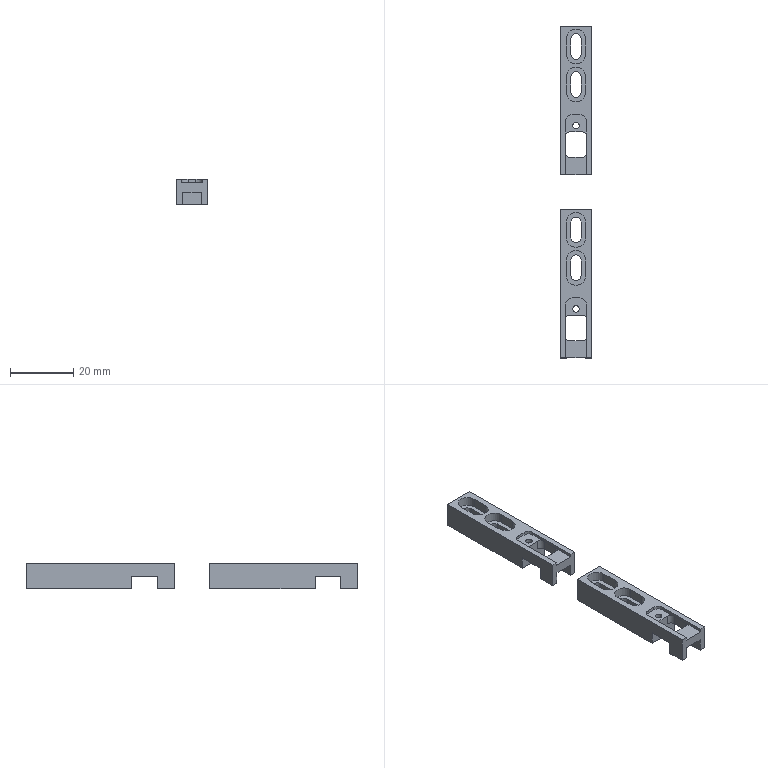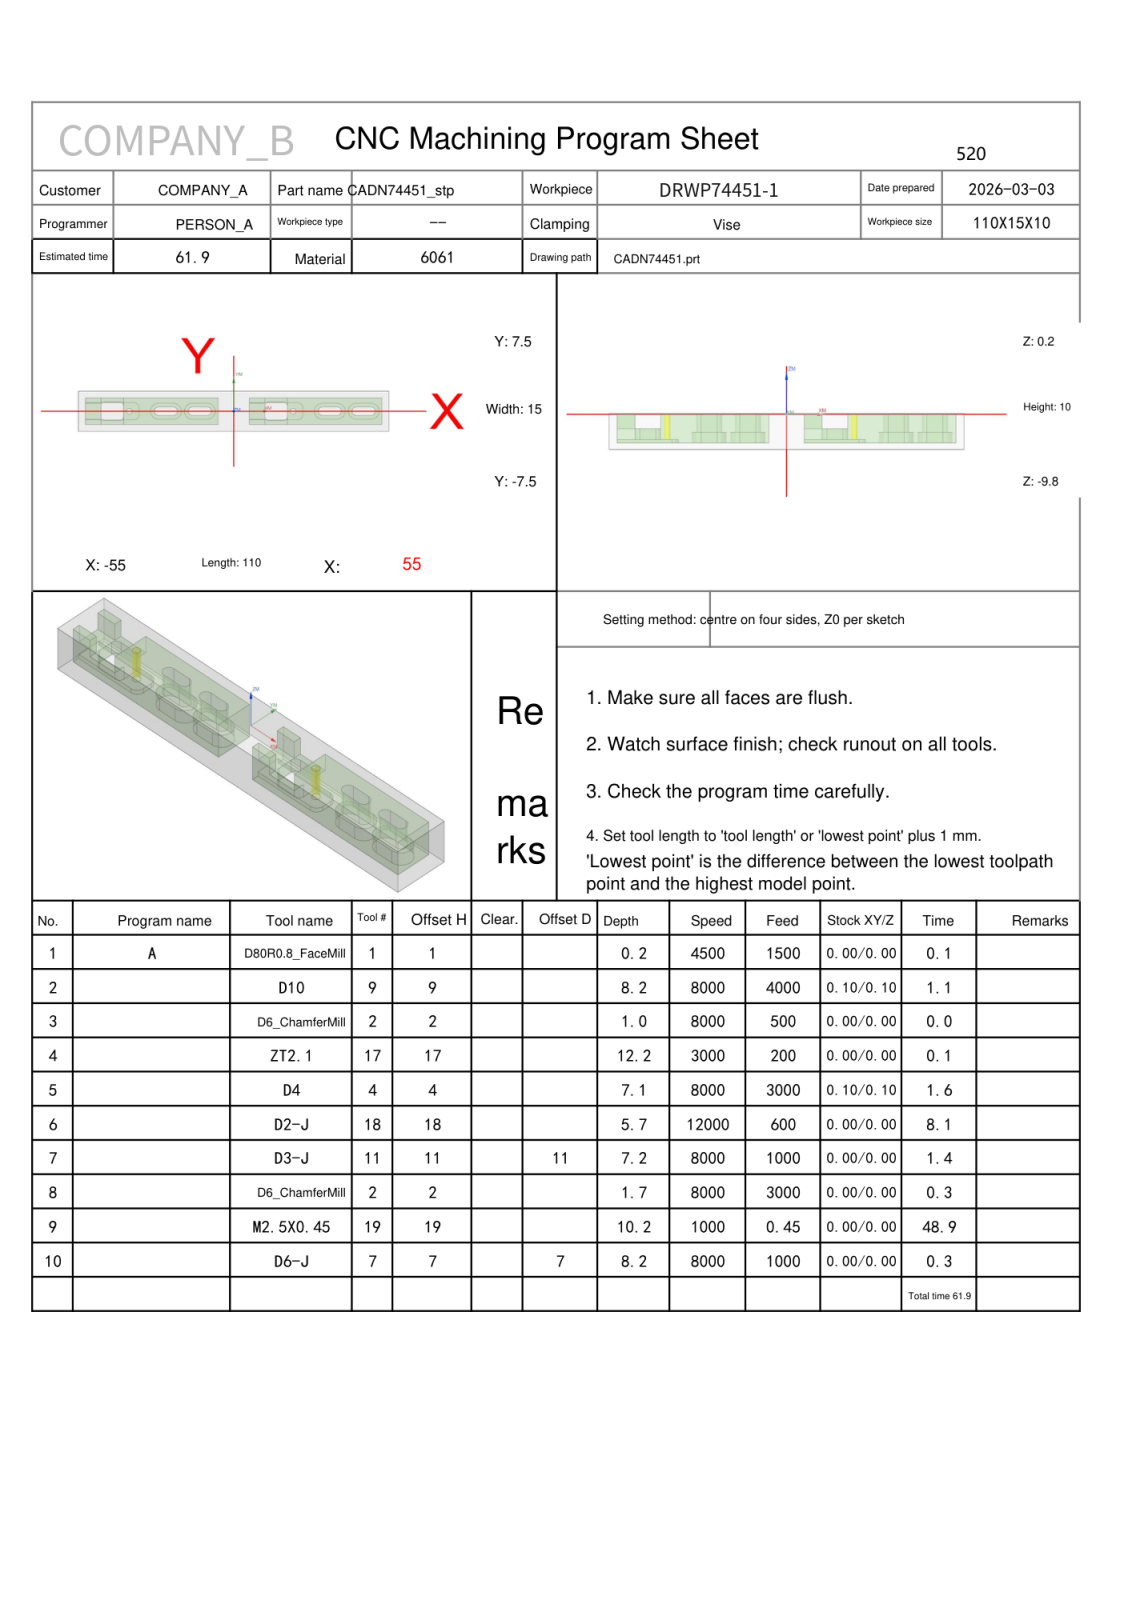NC program | NX | posted by the shop | part box 10 x 105 x 8 mm
Lines 4175 to 4761 of 4761:
N7 T11 M06
(D3-J  D=3. R=0. H=11 ce=0.00 di=0.00)
G00 G90 G54 X17.5 Y1.409 M03 S8000
G43 H11 Z50.
M08
Z.5
G01 Y2. Z.469 F600.
X12.5 Z.207
Y-1.95 Z0.0
G41 D11
Y-2.
X17.5 Z-.139
Y2. Z-.25
X12.5 Z-.389
Y-2. Z-.5
X17.5 Z-.639
Y2. Z-.75
X12.5 Z-.889
Y-2. Z-1.
X17.5 Z-1.139
Y2. Z-1.25
X12.5 Z-1.389
Y-2. Z-1.5
X17.5 Z-1.639
Y2. Z-1.75
X12.5 Z-1.889
Y-2. Z-2.
X17.5 Z-2.139
Y2. Z-2.25
X12.5 Z-2.389
Y-2. Z-2.5
X17.5 Z-2.639
Y2. Z-2.75
X12.5 Z-2.889
Y-2. Z-3.
X17.5 Z-3.139
Y2. Z-3.25
X12.5 Z-3.389
Y-2. Z-3.5
X17.5 Z-3.639
Y2. Z-3.75
X12.5 Z-3.889
Y-2. Z-4.
X17.5 Z-4.139
Y2. Z-4.25
X12.5 Z-4.389
Y-2. Z-4.5
X17.5 Z-4.639
Y2. Z-4.75
X12.5 Z-4.889
Y-2. Z-5.
X17.5 Z-5.139
Y2. Z-5.25
X12.5 Z-5.389
Y-2. Z-5.5
X17.5 Z-5.639
Y2. Z-5.75
X12.5 Z-5.889
Y-2. Z-6.
X17.5 Z-6.139
Y2. Z-6.25
X12.5 Z-6.389
Y-2. Z-6.5
X17.5 Z-6.639
Y2. Z-6.75
X12.5 Z-6.889
Y-2. Z-7.
X17.5
Y2.
X12.5
Y-2.
X12.9
X12.928 Y-1.998
X12.948 Y-1.978
X12.95 Y-1.95
G40 Y-1.9
Z-6.
G00 Z50.
X-45.5 Y-1.409
Z.5
G01 Y-2. Z.469
X-40.5 Z.207
Y1.95 Z0.0
G41 D11
Y2.
X-45.5 Z-.139
Y-2. Z-.25
X-40.5 Z-.389
Y2. Z-.5
X-45.5 Z-.639
Y-2. Z-.75
X-40.5 Z-.889
Y2. Z-1.
X-45.5 Z-1.139
Y-2. Z-1.25
X-40.5 Z-1.389
Y2. Z-1.5
X-45.5 Z-1.639
Y-2. Z-1.75
X-40.5 Z-1.889
Y2. Z-2.
X-45.5 Z-2.139
Y-2. Z-2.25
X-40.5 Z-2.389
Y2. Z-2.5
X-45.5 Z-2.639
Y-2. Z-2.75
X-40.5 Z-2.889
Y2. Z-3.
X-45.5 Z-3.139
Y-2. Z-3.25
X-40.5 Z-3.389
Y2. Z-3.5
X-45.5 Z-3.639
Y-2. Z-3.75
X-40.5 Z-3.889
Y2. Z-4.
X-45.5 Z-4.139
Y-2. Z-4.25
X-40.5 Z-4.389
Y2. Z-4.5
X-45.5 Z-4.639
Y-2. Z-4.75
X-40.5 Z-4.889
Y2. Z-5.
X-45.5 Z-5.139
Y-2. Z-5.25
X-40.5 Z-5.389
Y2. Z-5.5
X-45.5 Z-5.639
Y-2. Z-5.75
X-40.5 Z-5.889
Y2. Z-6.
X-45.5 Z-6.139
Y-2. Z-6.25
X-40.5 Z-6.389
Y2. Z-6.5
X-45.5 Z-6.639
Y-2. Z-6.75
X-40.5 Z-6.889
Y2. Z-7.
X-45.5
Y-2.
X-40.5
Y2.
X-40.9
X-40.928 Y1.998
X-40.948 Y1.978
X-40.95 Y1.95
G40 Y1.9
Z-6.
G00 Z50.
G00 G90 X-43. Y9.8 M03 S8000
Z50.
Z-3.5
G01 Z-4. F1000.
Y5.3
X-40.8
Y3.2
X-45.2
Y5.3
X-43.
X-42.5
Y9.8
Z-3.5
G00 Z50.
X-57.3 Y0.0
Z-3.5
G01 Z-4.
X-52.8
Y1.2
X-46.7
Y-1.2
X-52.8
Y0.0
Y.5
X-57.3
Z-3.5
G00 Z50.
X-43. Y-9.8
Z-3.5
G01 Z-4.
Y-5.3
X-45.2
Y-3.2
X-40.8
Y-5.3
X-43.
X-43.5
Y-9.8
Z-3.5
G00 Z50.
X15. Y9.8
Z-3.5
G01 Z-4.
Y5.3
X17.2
Y3.2
X12.8
Y5.3
X15.
X15.5
Y9.8
Z-3.5
G00 Z50.
X13.1
Z-3.5
G01 Z-4.
Y0.0
X11.3
Y-1.2
X5.2
Y1.2
X11.3
Y0.0
Y-.5
X13.1
Y-9.8
Z-3.5
G00 Z50.
X15.
Z-3.5
G01 Z-4.
Y-5.3
X12.8
Y-3.2
X17.2
Y-5.3
X15.
X14.5
Y-9.8
Z-3.5
G00 Z50.
G00 G90 X16.4 Y-7.35 M03 S8000
Z50.
Z-3.495
G01 Z-3.995 F1000.
G41 D11
X16.5
G03 X17.5 Y-6.35 I0.0 J1.
G01 Y6.35
G03 X16.5 Y7.35 I-1. J0.0
G01 G40 X16.4
Z-3.495
G00 Z50.
X13.6
Z-3.495
G01 Z-3.995
G41 D11
X13.5
G03 X12.5 Y6.35 I0.0 J-1.
G01 Y1.5
X4.15
G03 X3.15 Y.5 I0.0 J-1.
G01 G40 Y.4
Y-.4
G41 D11
Y-.5
G03 X4.15 Y-1.5 I1. J0.0
G01 X12.5
Y-6.35
G03 X13.5 Y-7.35 I1. J0.0
G01 G40 X13.6
Z-3.495
G00 Z50.
X-41.6
Z-3.495
G01 Z-3.995
G41 D11
X-41.5
G03 X-40.5 Y-6.35 I0.0 J1.
G01 Y6.35
G03 X-41.5 Y7.35 I-1. J0.0
G01 G40 X-41.6
Z-3.495
G00 Z50.
X-44.4
Z-3.495
G01 Z-3.995
G41 D11
X-44.5
G03 X-45.5 Y6.35 I0.0 J-1.
G01 Y1.5
X-53.85
G03 X-54.85 Y.5 I0.0 J-1.
G01 G40 Y.4
Y-.4
G41 D11
Y-.5
G03 X-53.85 Y-1.5 I1. J0.0
G01 X-45.5
Y-6.35
G03 X-44.5 Y-7.35 I1. J0.0
G01 G40 X-44.4
Z-3.495
G00 Z50.
G91 G28 Z0.0
M05
M09
G91 G28 Z0.0
M01
N8 T02 M06
(D6_ChamferMill  D=6. R=0. H=02 ce=0.00 di=0.00)
G00 G90 G54 X36. Y-7.128 M03 S8000
G43 H02 Z50.
M08
Z2.099
G01 Z-1.5 F3000.
G03 X36.08 Y-6.828 I-.52 J.3
X35.78 Y-6.308 I-.6 J0.0
G01 X35.75 Y-6.3
X19.
G02 X17.7 Y-5. I0.0 J1.3
G01 Y5.
G02 X19. Y6.3 I1.3 J0.0
G01 X52.5
G02 X53.8 Y5. I0.0 J-1.3
G01 Y-5.
G02 X52.5 Y-6.3 I-1.3 J0.0
G01 X35.75
X35.72 Y-6.308
G03 X35.42 Y-6.828 I.3 J-.52
X35.5 Y-7.128 I.6 J0.0
G01 Z2.099
G00 Z6.
X33.8 Y.362
Z2.985
G01 Z-1.5
G03 X33.736 Y.122 I.416 J-.24
X33.976 Y-.294 I.48 J0.0
G01 X34. Y-.3
X36.5
G03 X36.8 Y0.0 I0.0 J.3
G01 X36.777 Y.115
X36.712 Y.212
X36.615 Y.277
X36.5 Y.3
X31.5
G03 X31.2 Y0.0 I0.0 J-.3
G01 X31.223 Y-.115
X31.288 Y-.212
X31.385 Y-.277
X31.5 Y-.3
X34.
X34.024 Y-.294
G03 X34.264 Y.122 I-.24 J.416
X34.2 Y.362 I-.48 J0.0
G01 Z2.985
G00 Z50.
X46.2 Y-.362
Z2.985
G01 Z-1.5
G03 X46.264 Y-.122 I-.416 J.24
X46.024 Y.294 I-.48 J0.0
G01 X46. Y.3
X43.5
G03 X43.2 Y0.0 I0.0 J-.3
G01 X43.223 Y-.115
X43.288 Y-.212
X43.385 Y-.277
X43.5 Y-.3
X48.5
G03 X48.8 Y0.0 I0.0 J.3
G01 X48.777 Y.115
X48.712 Y.212
X48.615 Y.277
X48.5 Y.3
X46.
X45.976 Y.294
G03 X45.736 Y-.122 I.24 J-.416
X45.8 Y-.362 I.48 J0.0
G01 Z2.985
G00 Z50.
X8.5 Y.872
Z2.099
G01 Z-1.5
G03 X8.58 Y1.172 I-.52 J.3
X8.28 Y1.692 I-.6 J0.0
G01 X8.25 Y1.7
X5.5
G02 X4.2 Y3. I0.0 J1.3
G01 Y5.
G02 X5.5 Y6.3 I1.3 J0.0
G01 X11.
G02 X12.3 Y5. I0.0 J-1.3
G01 Y3.
G02 X11. Y1.7 I-1.3 J0.0
G01 X8.25
X8.22 Y1.692
G03 X7.92 Y1.172 I.3 J-.52
X8. Y.872 I.6 J0.0
G01 Z2.099
G00 Z2.25
Y-.872
Z2.099
G01 Z-1.5
G03 X7.92 Y-1.172 I.52 J-.3
X8.22 Y-1.692 I.6 J0.0
G01 X8.25 Y-1.7
X11.
G02 X12.3 Y-3. I0.0 J-1.3
G01 Y-5.
G02 X11. Y-6.3 I-1.3 J0.0
G01 X5.5
G02 X4.2 Y-5. I0.0 J1.3
G01 Y-3.
G02 X5.5 Y-1.7 I1.3 J0.0
G01 X8.25
X8.28 Y-1.692
G03 X8.58 Y-1.172 I-.3 J.52
X8.5 Y-.872 I-.6 J0.0
G01 Z2.099
G00 Z50.
X-22. Y-7.128
Z2.099
G01 Z-1.5
G03 X-21.92 Y-6.828 I-.52 J.3
X-22.22 Y-6.308 I-.6 J0.0
G01 X-22.25 Y-6.3
X-39.
G02 X-40.3 Y-5. I0.0 J1.3
G01 Y5.
G02 X-39. Y6.3 I1.3 J0.0
G01 X-5.5
G02 X-4.2 Y5. I0.0 J-1.3
G01 Y-5.
G02 X-5.5 Y-6.3 I-1.3 J0.0
G01 X-22.25
X-22.28 Y-6.308
G03 X-22.58 Y-6.828 I.3 J-.52
X-22.5 Y-7.128 I.6 J0.0
G01 Z2.099
G00 Z6.
X-23.8 Y-.362
Z2.985
G01 Z-1.5
G03 X-23.736 Y-.122 I-.416 J.24
X-23.976 Y.294 I-.48 J0.0
G01 X-24. Y.3
X-26.5
G03 X-26.8 Y0.0 I0.0 J-.3
G01 X-26.777 Y-.115
X-26.712 Y-.212
X-26.615 Y-.277
X-26.5 Y-.3
X-21.5
G03 X-21.2 Y0.0 I0.0 J.3
G01 X-21.223 Y.115
X-21.288 Y.212
X-21.385 Y.277
X-21.5 Y.3
X-24.
X-24.024 Y.294
G03 X-24.264 Y-.122 I.24 J-.416
X-24.2 Y-.362 I.48 J0.0
G01 Z2.985
G00 Z50.
X-12.2 Y.362
Z2.985
G01 Z-1.5
G03 X-12.264 Y.122 I.416 J-.24
X-12.024 Y-.294 I.48 J0.0
G01 X-12. Y-.3
X-9.5
G03 X-9.2 Y0.0 I0.0 J.3
G01 X-9.223 Y.115
X-9.288 Y.212
X-9.385 Y.277
X-9.5 Y.3
X-14.5
G03 X-14.8 Y0.0 I0.0 J-.3
G01 X-14.777 Y-.115
X-14.712 Y-.212
X-14.615 Y-.277
X-14.5 Y-.3
X-12.
X-11.976 Y-.294
G03 X-11.736 Y.122 I-.24 J.416
X-11.8 Y.362 I-.48 J0.0
G01 Z2.985
G00 Z50.
X-50. Y7.128
Z2.099
G01 Z-1.5
G03 X-50.08 Y6.828 I.52 J-.3
X-49.78 Y6.308 I.6 J0.0
G01 X-49.75 Y6.3
X-47.
G02 X-45.7 Y5. I0.0 J-1.3
G01 Y3.
G02 X-47. Y1.7 I-1.3 J0.0
G01 X-52.5
G02 X-53.8 Y3. I0.0 J1.3
G01 Y5.
G02 X-52.5 Y6.3 I1.3 J0.0
G01 X-49.75
X-49.72 Y6.308
G03 X-49.42 Y6.828 I-.3 J.52
X-49.5 Y7.128 I-.6 J0.0
G01 Z2.099
G00 Z50.
Y-7.128
Z2.099
G01 Z-1.5
G03 X-49.42 Y-6.828 I-.52 J.3
X-49.72 Y-6.308 I-.6 J0.0
G01 X-49.75 Y-6.3
X-52.5
G02 X-53.8 Y-5. I0.0 J1.3
G01 Y-3.
G02 X-52.5 Y-1.7 I1.3 J0.0
G01 X-47.
G02 X-45.7 Y-3. I0.0 J-1.3
G01 Y-5.
G02 X-47. Y-6.3 I-1.3 J0.0
G01 X-49.75
X-49.78 Y-6.308
G03 X-50.08 Y-6.828 I.3 J-.52
X-50. Y-7.128 I.6 J0.0
G01 Z2.099
G00 Z50.
G00 G90 X21. Y0.0 M03 S8000
Z50.
G98 G81 X21. Y0.0 Z-1.475 R3. F500.
X-37.
G80
G00 Z50.
G91 G28 Z0.0
M05
M09
G91 G28 Z0.0
M01
N9 T19 M06
(M2.5X0.45 D=2.05 DR_a=180 H=19)
G00 G90 G54 X21. Y0.0 M03 S1000
G43 H19 Z50.
M08
G95
G98 G84 X21. Y0.0 Z-10. R1. F.45 Q5.
X-37.
G80
G94
G00 Z50.
G91 G28 Z0.0
M05
M09
G91 G28 Z0.0
M01
N10 T07 M06
(D6-J  D=6. R=0. H=07 ce=0.00 di=0.00)
G00 G90 G54 X56.4 Y-9.1 M03 S8000
G43 H07 Z10.2
M08
Z-6.5
G01 Z-8. F1000.
G41 D07
Y-8.9
G03 X55.5 Y-8. I-.9 J0.0
G01 X2.5
Y8.
X55.5
Y-8.
X55.1
G03 X54.2 Y-8.9 I0.0 J-.9
G01 G40 Y-9.1
Z-6.5
G00 X-28.1
G01 Z-8.
G41 D07
Y-8.9
G03 X-29. Y-8. I-.9 J0.0
G01 X-55.5
Y8.
X-2.5
Y-8.
X-29.
X-29.4
G03 X-30.3 Y-8.9 I0.0 J-.9
G01 G40 Y-9.1
Z-6.5
G00 Z10.2
M05
M09
G91 G28 Z0.0
G91 G28 Y0.0
M30
%